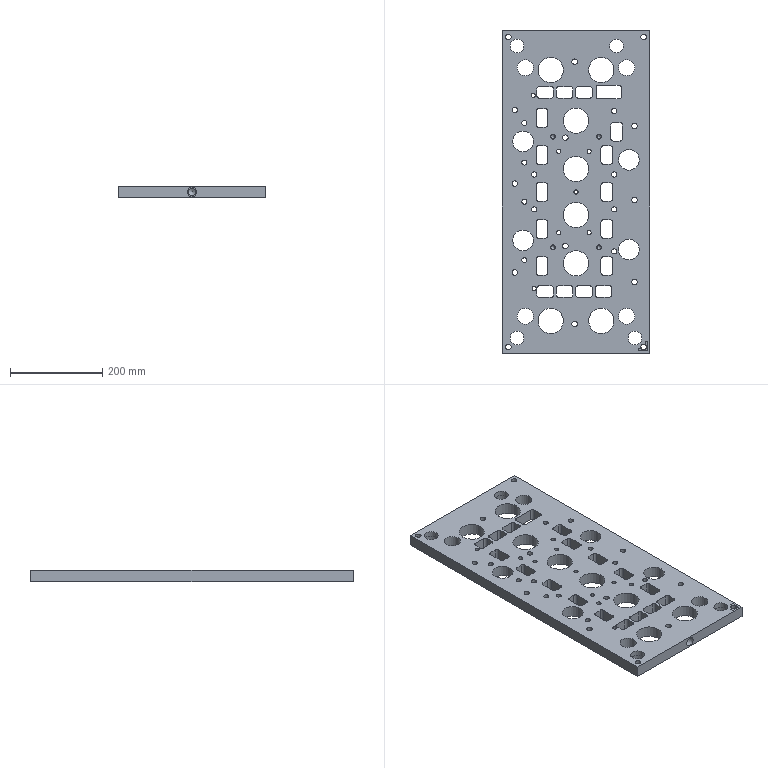Part | STEP file | DZMB | 1 solid | 291 faces | box 320 x 700 x 25 mm | volume 4227147 mm3 | cylinder 156 | plane 129 | cone 6 | commonest cylinder face diameters 10 x76 12 x14 9 x11 11 x10 16 x10 55 x8